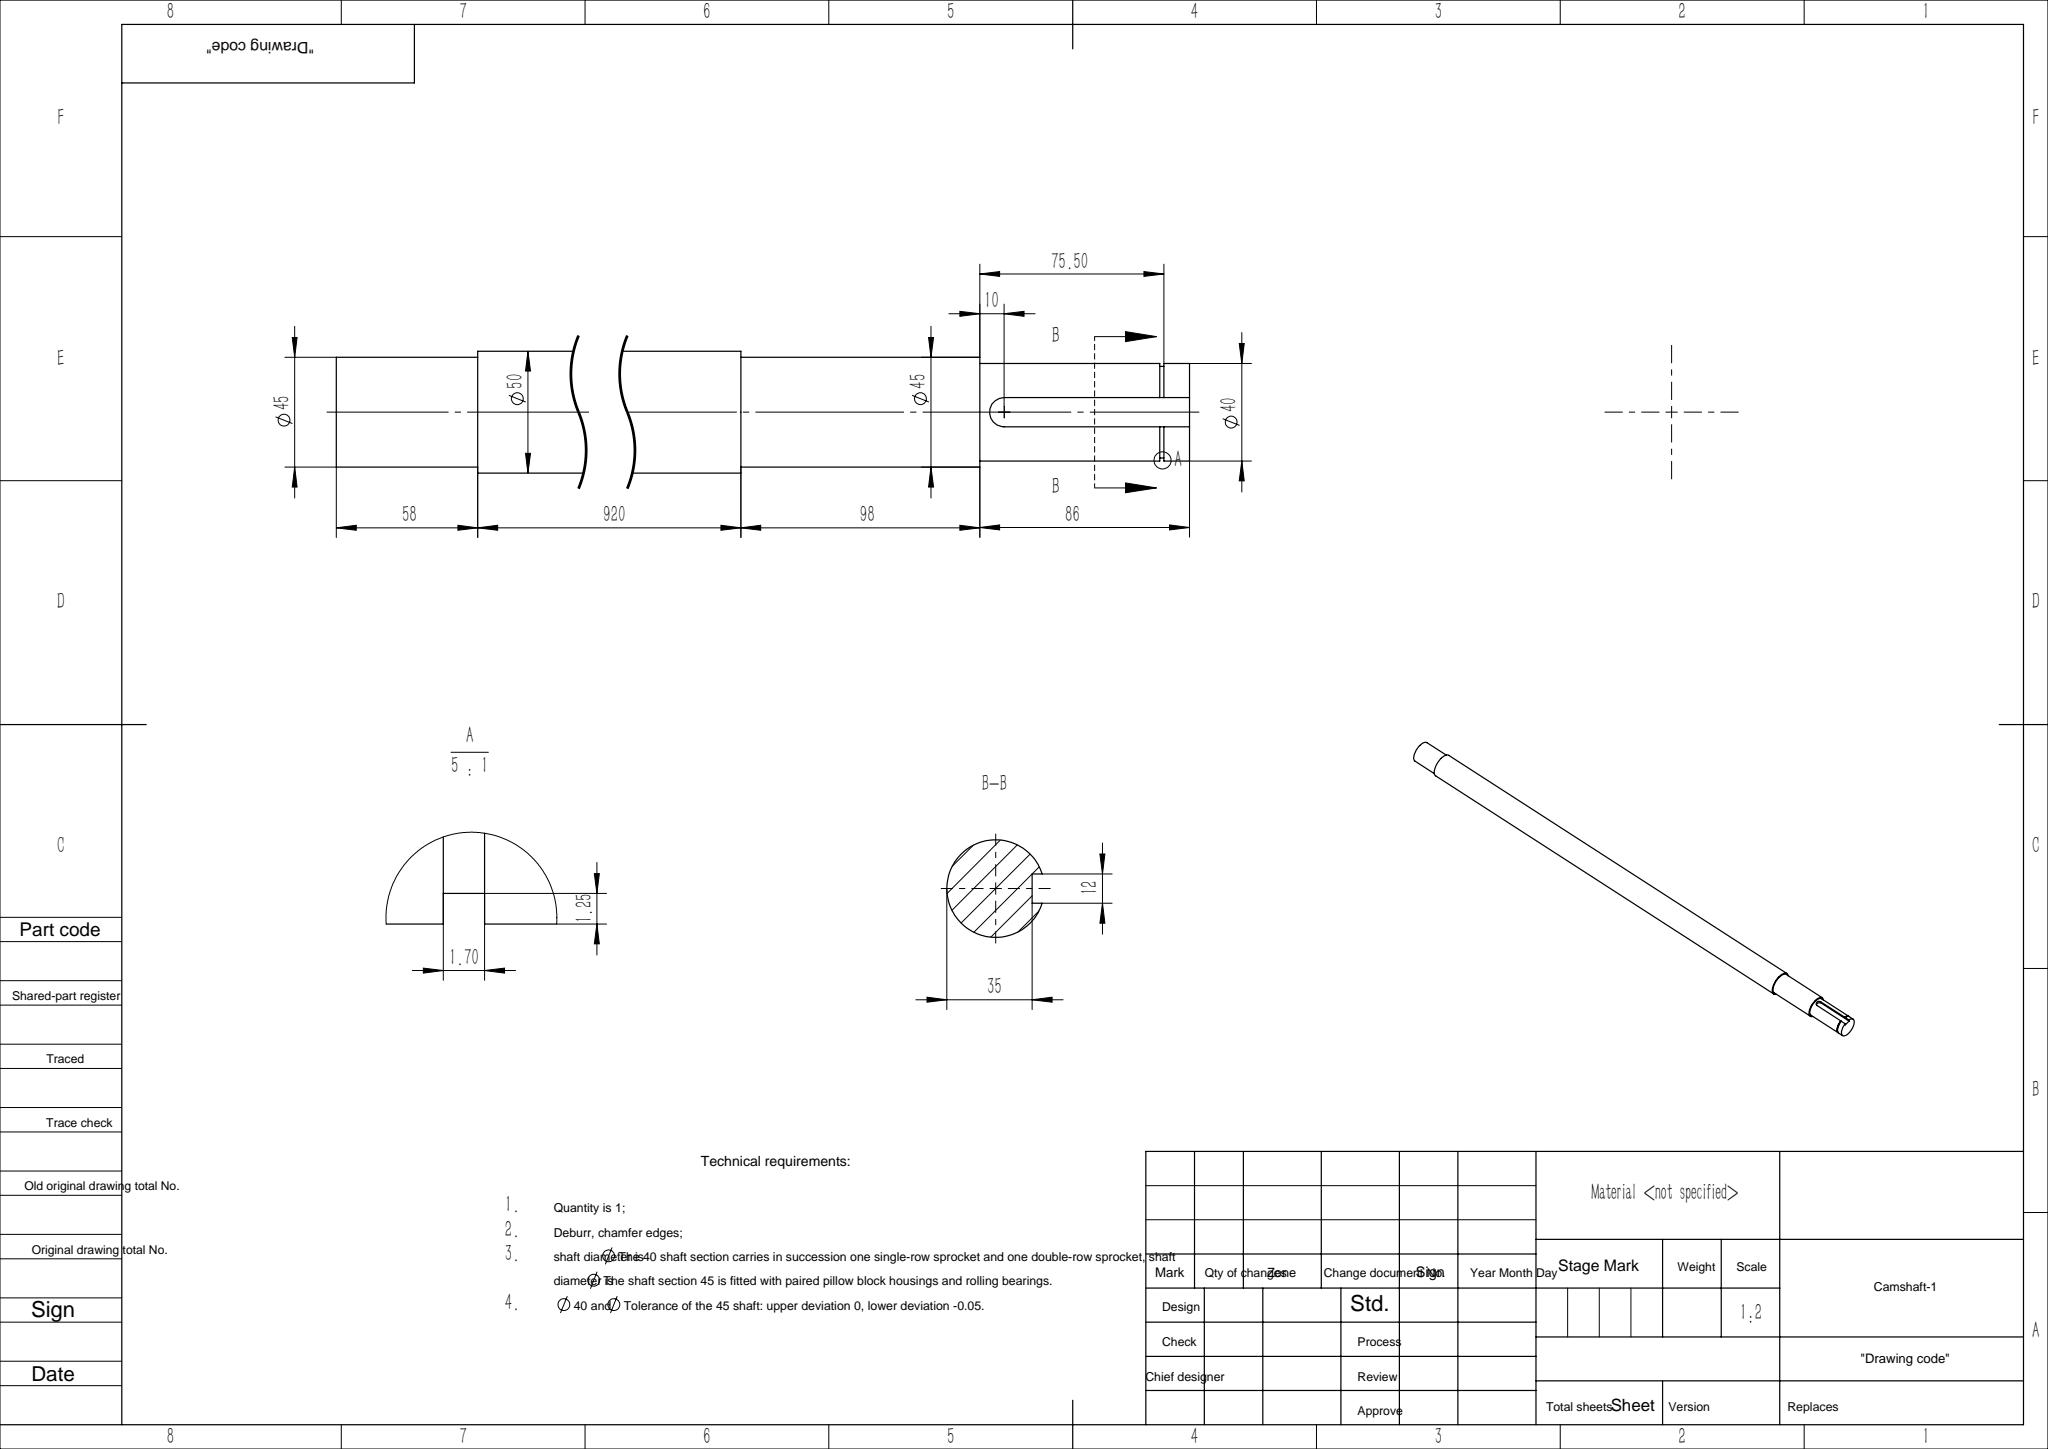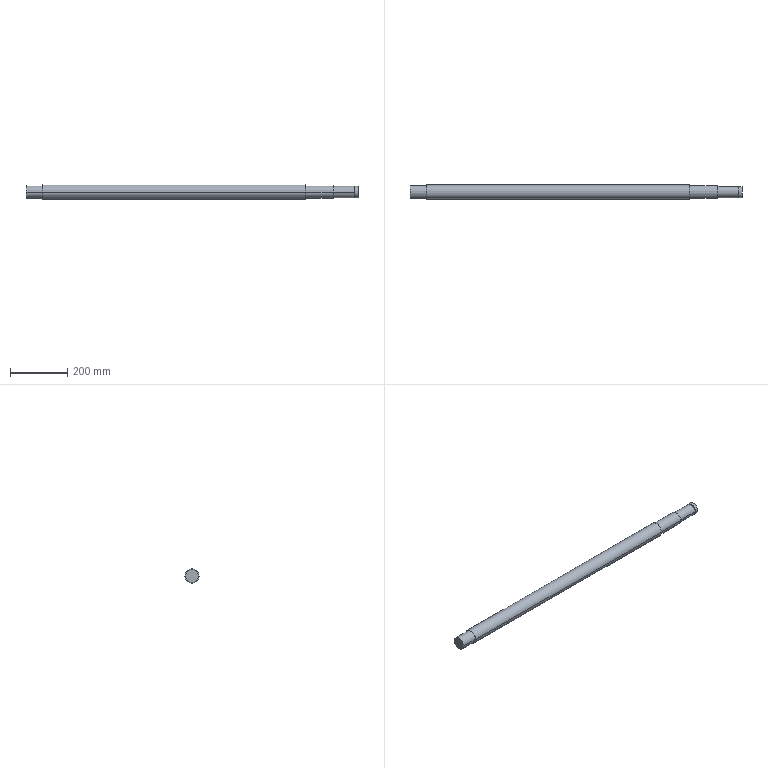Part | SolidWorks | features ICE 2, Revolution 1 | 1 solid | 22 faces | box 1162 x 50 x 50 mm | volume 2157809 mm3 | cylinder 12 | plane 10 | commonest cylinder face diameters 45 x4 40 x3 12 x2 50 x2 37.5 x1
STEP:
#1=CARTESIAN_POINT('',(1080.,15.,0.));
#2=VERTEX_POINT('',#1);
#3=CARTESIAN_POINT('',(1086.,15.,6.));
#4=VERTEX_POINT('',#3);
#5=CARTESIAN_POINT('',(1086.,15.,0.));
#6=DIRECTION('',(0.,1.,0.));
#7=DIRECTION('',(-1.,0.,0.));
#8=AXIS2_PLACEMENT_3D('',#5,#6,#7);
#9=CIRCLE('',#8,6.);
#10=EDGE_CURVE('',#2,#4,#9,.T.);
#11=ORIENTED_EDGE('',*,*,#10,.F.);
#12=CARTESIAN_POINT('',(1080.,20.,0.));
#13=VERTEX_POINT('',#12);
#14=CARTESIAN_POINT('',(1080.,15.,0.));
#15=DIRECTION('',(0.,1.,0.));
#16=VECTOR('',#15,1000.);
#17=LINE('',#14,#16);
#18=EDGE_CURVE('',#2,#13,#17,.T.);
#19=ORIENTED_EDGE('',*,*,#18,.T.);
#20=CARTESIAN_POINT('',(1086.,19.079,6.));
#21=VERTEX_POINT('',#20);
#22=CARTESIAN_POINT('',(1080.,20.,0.));
#23=CARTESIAN_POINT('',(1080.,20.,0.3936));
#24=CARTESIAN_POINT('',(1080.04,19.988,0.7934));
#25=CARTESIAN_POINT('',(1080.194,19.942,1.564));
#26=CARTESIAN_POINT('',(1080.308,19.909,1.939));
#27=CARTESIAN_POINT('',(1080.611,19.825,2.668));
#28=CARTESIAN_POINT('',(1080.798,19.774,3.015));
#29=CARTESIAN_POINT('',(1081.123,19.692,3.5));
#30=CARTESIAN_POINT('',(1081.239,19.664,3.657));
#31=CARTESIAN_POINT('',(1081.487,19.605,3.959));
#32=CARTESIAN_POINT('',(1081.62,19.575,4.105));
#33=CARTESIAN_POINT('',(1082.035,19.485,4.52));
#34=CARTESIAN_POINT('',(1082.335,19.425,4.766));
#35=CARTESIAN_POINT('',(1082.982,19.313,5.201));
#36=CARTESIAN_POINT('',(1083.333,19.261,5.389));
#37=CARTESIAN_POINT('',(1084.055,19.174,5.69));
#38=CARTESIAN_POINT('',(1084.429,19.139,5.804));
#39=CARTESIAN_POINT('',(1085.203,19.092,5.96));
#40=CARTESIAN_POINT('',(1085.601,19.079,6.));
#41=CARTESIAN_POINT('',(1086.,19.079,6.));
#42=B_SPLINE_CURVE_WITH_KNOTS('',3,(#22,#23,#24,#25,#26,#27,#28,#29,#30,#31,#32,#33,#34,#35,#36,#37,#38,#39,#40,#41),.UNSPECIFIED.,.F.,.F.,(4,2,2,2,2,2,2,2,2,4),(0.009436,0.01061,0.01179,0.01297,0.01356,0.01415,0.01533,0.0165,0.01768,0.01886),.UNSPECIFIED.);
#43=EDGE_CURVE('',#13,#21,#42,.T.);
#44=ORIENTED_EDGE('',*,*,#43,.T.);
#45=CARTESIAN_POINT('',(1086.,15.,6.));
#46=DIRECTION('',(0.,1.,0.));
#47=VECTOR('',#46,1000.);
#48=LINE('',#45,#47);
#49=EDGE_CURVE('',#4,#21,#48,.T.);
#50=ORIENTED_EDGE('',*,*,#49,.F.);
#51=EDGE_LOOP('',(#11,#19,#44,#50));
#52=FACE_OUTER_BOUND('',#51,.T.);
#53=CARTESIAN_POINT('',(1086.,15.,0.));
#54=DIRECTION('',(0.,1.,0.));
#55=DIRECTION('',(-1.,0.,0.));
#56=AXIS2_PLACEMENT_3D('',#53,#54,#55);
#57=CYLINDRICAL_SURFACE('',#56,6.);
#58=ADVANCED_FACE('',(#52),#57,.F.);
#59=CARTESIAN_POINT('',(978.,22.5,0.));
#60=VERTEX_POINT('',#59);
#61=CARTESIAN_POINT('',(978.,-22.5,0.));
#62=VERTEX_POINT('',#61);
#63=CARTESIAN_POINT('',(978.,0.,0.));
#64=DIRECTION('',(1.,0.,0.));
#65=DIRECTION('',(0.,1.,0.));
#66=AXIS2_PLACEMENT_3D('',#63,#64,#65);
#67=CIRCLE('',#66,22.5);
#68=EDGE_CURVE('',#60,#62,#67,.T.);
#69=ORIENTED_EDGE('',*,*,#68,.T.);
#70=CARTESIAN_POINT('',(1076.,-22.5,0.));
#71=VERTEX_POINT('',#70);
#72=CARTESIAN_POINT('',(1162.,-22.5,0.));
#73=DIRECTION('',(1.,0.,0.));
#74=VECTOR('',#73,1000.);
#75=LINE('',#72,#74);
#76=EDGE_CURVE('',#62,#71,#75,.T.);
#77=ORIENTED_EDGE('',*,*,#76,.T.);
#78=CARTESIAN_POINT('',(1076.,22.5,0.));
#79=VERTEX_POINT('',#78);
#80=CARTESIAN_POINT('',(1076.,0.,0.));
#81=DIRECTION('',(1.,0.,0.));
#82=DIRECTION('',(0.,1.,0.));
#83=AXIS2_PLACEMENT_3D('',#80,#81,#82);
#84=CIRCLE('',#83,22.5);
#85=EDGE_CURVE('',#79,#71,#84,.T.);
#86=ORIENTED_EDGE('',*,*,#85,.F.);
#87=CARTESIAN_POINT('',(1162.,22.5,0.));
#88=DIRECTION('',(1.,0.,0.));
#89=VECTOR('',#88,1000.);
#90=LINE('',#87,#89);
#91=EDGE_CURVE('',#60,#79,#90,.T.);
#92=ORIENTED_EDGE('',*,*,#91,.F.);
#93=EDGE_LOOP('',(#69,#77,#86,#92));
#94=FACE_OUTER_BOUND('',#93,.T.);
#95=CARTESIAN_POINT('',(1162.,0.,0.));
#96=DIRECTION('',(1.,0.,0.));
#97=DIRECTION('',(0.,1.,0.));
#98=AXIS2_PLACEMENT_3D('',#95,#96,#97);
#99=CYLINDRICAL_SURFACE('',#98,22.5);
#100=ADVANCED_FACE('',(#94),#99,.T.);
#101=CARTESIAN_POINT('',(58.,25.,0.));
#102=VERTEX_POINT('',#101);
#103=CARTESIAN_POINT('',(58.,-25.,0.));
#104=VERTEX_POINT('',#103);
#105=CARTESIAN_POINT('',(58.,0.,0.));
#106=DIRECTION('',(1.,0.,0.));
#107=DIRECTION('',(0.,1.,0.));
#108=AXIS2_PLACEMENT_3D('',#105,#106,#107);
#109=CIRCLE('',#108,25.);
#110=EDGE_CURVE('',#102,#104,#109,.T.);
#111=ORIENTED_EDGE('',*,*,#110,.T.);
#112=CARTESIAN_POINT('',(978.,-25.,0.));
#113=VERTEX_POINT('',#112);
#114=CARTESIAN_POINT('',(1162.,-25.,0.));
#115=DIRECTION('',(1.,0.,0.));
#116=VECTOR('',#115,1000.);
#117=LINE('',#114,#116);
#118=EDGE_CURVE('',#104,#113,#117,.T.);
#119=ORIENTED_EDGE('',*,*,#118,.T.);
#120=CARTESIAN_POINT('',(978.,25.,0.));
#121=VERTEX_POINT('',#120);
#122=CARTESIAN_POINT('',(978.,0.,0.));
#123=DIRECTION('',(1.,0.,0.));
#124=DIRECTION('',(0.,1.,0.));
#125=AXIS2_PLACEMENT_3D('',#122,#123,#124);
#126=CIRCLE('',#125,25.);
#127=EDGE_CURVE('',#121,#113,#126,.T.);
#128=ORIENTED_EDGE('',*,*,#127,.F.);
#129=CARTESIAN_POINT('',(1162.,25.,0.));
#130=DIRECTION('',(1.,0.,0.));
#131=VECTOR('',#130,1000.);
#132=LINE('',#129,#131);
#133=EDGE_CURVE('',#102,#121,#132,.T.);
#134=ORIENTED_EDGE('',*,*,#133,.F.);
#135=EDGE_LOOP('',(#111,#119,#128,#134));
#136=FACE_OUTER_BOUND('',#135,.T.);
#137=CARTESIAN_POINT('',(1162.,0.,0.));
#138=DIRECTION('',(1.,0.,0.));
#139=DIRECTION('',(0.,1.,0.));
#140=AXIS2_PLACEMENT_3D('',#137,#138,#139);
#141=CYLINDRICAL_SURFACE('',#140,25.);
#142=ADVANCED_FACE('',(#136),#141,.T.);
#143=CARTESIAN_POINT('',(0.,22.5,0.));
#144=VERTEX_POINT('',#143);
#145=CARTESIAN_POINT('',(0.,-22.5,0.));
#146=VERTEX_POINT('',#145);
#147=CARTESIAN_POINT('',(0.,0.,0.));
#148=DIRECTION('',(1.,0.,0.));
#149=DIRECTION('',(0.,1.,0.));
#150=AXIS2_PLACEMENT_3D('',#147,#148,#149);
#151=CIRCLE('',#150,22.5);
#152=EDGE_CURVE('',#144,#146,#151,.T.);
#153=ORIENTED_EDGE('',*,*,#152,.T.);
#154=CARTESIAN_POINT('',(58.,-22.5,0.));
#155=VERTEX_POINT('',#154);
#156=CARTESIAN_POINT('',(1162.,-22.5,0.));
#157=DIRECTION('',(1.,0.,0.));
#158=VECTOR('',#157,1000.);
#159=LINE('',#156,#158);
#160=EDGE_CURVE('',#146,#155,#159,.T.);
#161=ORIENTED_EDGE('',*,*,#160,.T.);
#162=CARTESIAN_POINT('',(58.,22.5,0.));
#163=VERTEX_POINT('',#162);
#164=CARTESIAN_POINT('',(58.,0.,0.));
#165=DIRECTION('',(1.,0.,0.));
#166=DIRECTION('',(0.,1.,0.));
#167=AXIS2_PLACEMENT_3D('',#164,#165,#166);
#168=CIRCLE('',#167,22.5);
#169=EDGE_CURVE('',#163,#155,#168,.T.);
#170=ORIENTED_EDGE('',*,*,#169,.F.);
#171=CARTESIAN_POINT('',(1162.,22.5,0.));
#172=DIRECTION('',(1.,0.,0.));
#173=VECTOR('',#172,1000.);
#174=LINE('',#171,#173);
#175=EDGE_CURVE('',#144,#163,#174,.T.);
#176=ORIENTED_EDGE('',*,*,#175,.F.);
#177=EDGE_LOOP('',(#153,#161,#170,#176));
#178=FACE_OUTER_BOUND('',#177,.T.);
#179=CARTESIAN_POINT('',(1162.,0.,0.));
#180=DIRECTION('',(1.,0.,0.));
#181=DIRECTION('',(0.,1.,0.));
#182=AXIS2_PLACEMENT_3D('',#179,#180,#181);
#183=CYLINDRICAL_SURFACE('',#182,22.5);
#184=ADVANCED_FACE('',(#178),#183,.T.);
#185=CARTESIAN_POINT('',(1076.,20.,0.));
#186=VERTEX_POINT('',#185);
#187=CARTESIAN_POINT('',(1076.,-20.,0.));
#188=VERTEX_POINT('',#187);
#189=CARTESIAN_POINT('',(1076.,0.,0.));
#190=DIRECTION('',(1.,0.,0.));
#191=DIRECTION('',(0.,1.,0.));
#192=AXIS2_PLACEMENT_3D('',#189,#190,#191);
#193=CIRCLE('',#192,20.);
#194=EDGE_CURVE('',#186,#188,#193,.T.);
#195=ORIENTED_EDGE('',*,*,#194,.T.);
#196=CARTESIAN_POINT('',(1149.8,-20.,0.));
#197=VERTEX_POINT('',#196);
#198=CARTESIAN_POINT('',(1162.,-20.,0.));
#199=DIRECTION('',(1.,0.,0.));
#200=VECTOR('',#199,1000.);
#201=LINE('',#198,#200);
#202=EDGE_CURVE('',#188,#197,#201,.T.);
#203=ORIENTED_EDGE('',*,*,#202,.T.);
#204=CARTESIAN_POINT('',(1149.8,19.079,6.));
#205=VERTEX_POINT('',#204);
#206=CARTESIAN_POINT('',(1149.8,0.,0.));
#207=DIRECTION('',(1.,0.,0.));
#208=DIRECTION('',(0.,1.,0.));
#209=AXIS2_PLACEMENT_3D('',#206,#207,#208);
#210=CIRCLE('',#209,20.);
#211=EDGE_CURVE('',#205,#197,#210,.T.);
#212=ORIENTED_EDGE('',*,*,#211,.F.);
#213=CARTESIAN_POINT('',(1162.,19.079,6.));
#214=DIRECTION('',(1.,0.,0.));
#215=VECTOR('',#214,1000.);
#216=LINE('',#213,#215);
#217=EDGE_CURVE('',#21,#205,#216,.T.);
#218=ORIENTED_EDGE('',*,*,#217,.F.);
#219=ORIENTED_EDGE('',*,*,#43,.F.);
#220=CARTESIAN_POINT('',(1162.,20.,0.));
#221=DIRECTION('',(1.,0.,0.));
#222=VECTOR('',#221,1000.);
#223=LINE('',#220,#222);
#224=EDGE_CURVE('',#186,#13,#223,.T.);
#225=ORIENTED_EDGE('',*,*,#224,.F.);
#226=EDGE_LOOP('',(#195,#203,#212,#218,#219,#225));
#227=FACE_OUTER_BOUND('',#226,.T.);
#228=CARTESIAN_POINT('',(1162.,0.,0.));
#229=DIRECTION('',(1.,0.,0.));
#230=DIRECTION('',(0.,1.,0.));
#231=AXIS2_PLACEMENT_3D('',#228,#229,#230);
#232=CYLINDRICAL_SURFACE('',#231,20.);
#233=ADVANCED_FACE('',(#227),#232,.T.);
#234=ORIENTED_EDGE('',*,*,#202,.F.);
#235=CARTESIAN_POINT('',(1076.,0.,0.));
#236=DIRECTION('',(1.,0.,0.));
#237=DIRECTION('',(0.,1.,0.));
#238=AXIS2_PLACEMENT_3D('',#235,#236,#237);
#239=CIRCLE('',#238,20.);
#240=EDGE_CURVE('',#188,#186,#239,.T.);
#241=ORIENTED_EDGE('',*,*,#240,.T.);
#242=ORIENTED_EDGE('',*,*,#224,.T.);
#243=CARTESIAN_POINT('',(1086.,19.079,-6.));
#244=VERTEX_POINT('',#243);
#245=CARTESIAN_POINT('',(1086.,19.079,-6.));
#246=CARTESIAN_POINT('',(1085.601,19.079,-6.));
#247=CARTESIAN_POINT('',(1085.209,19.091,-5.961));
#248=CARTESIAN_POINT('',(1084.631,19.127,-5.845));
#249=CARTESIAN_POINT('',(1084.441,19.141,-5.797));
#250=CARTESIAN_POINT('',(1084.062,19.176,-5.682));
#251=CARTESIAN_POINT('',(1083.875,19.196,-5.615));
#252=CARTESIAN_POINT('',(1083.331,19.261,-5.388));
#253=CARTESIAN_POINT('',(1082.987,19.313,-5.203));
#254=CARTESIAN_POINT('',(1082.499,19.397,-4.877));
#255=CARTESIAN_POINT('',(1082.34,19.426,-4.759));
#256=CARTESIAN_POINT('',(1082.037,19.485,-4.51));
#257=CARTESIAN_POINT('',(1081.893,19.515,-4.378));
#258=CARTESIAN_POINT('',(1081.481,19.605,-3.966));
#259=CARTESIAN_POINT('',(1081.233,19.664,-3.665));
#260=CARTESIAN_POINT('',(1080.794,19.775,-3.009));
#261=CARTESIAN_POINT('',(1080.609,19.825,-2.664));
#262=CARTESIAN_POINT('',(1080.385,19.888,-2.122));
#263=CARTESIAN_POINT('',(1080.318,19.907,-1.938));
#264=CARTESIAN_POINT('',(1080.203,19.94,-1.561));
#265=CARTESIAN_POINT('',(1080.154,19.954,-1.367));
#266=CARTESIAN_POINT('',(1080.038,19.988,-0.7852));
#267=CARTESIAN_POINT('',(1080.,20.,-0.3941));
#268=CARTESIAN_POINT('',(1080.,20.,0.));
#269=B_SPLINE_CURVE_WITH_KNOTS('',3,(#245,#246,#247,#248,#249,#250,#251,#252,#253,#254,#255,#256,#257,#258,#259,#260,#261,#262,#263,#264,#265,#266,#267,#268),.UNSPECIFIED.,.F.,.F.,(4,2,2,2,2,2,2,2,2,2,2,4),(0.,0.00118,0.001769,0.002359,0.003539,0.004128,0.004718,0.005898,0.007077,0.007667,0.008257,0.009436),.UNSPECIFIED.);
#270=EDGE_CURVE('',#244,#13,#269,.T.);
#271=ORIENTED_EDGE('',*,*,#270,.F.);
#272=CARTESIAN_POINT('',(1149.8,19.079,-6.));
#273=VERTEX_POINT('',#272);
#274=CARTESIAN_POINT('',(1162.,19.079,-6.));
#275=DIRECTION('',(-1.,0.,0.));
#276=VECTOR('',#275,1000.);
#277=LINE('',#274,#276);
#278=EDGE_CURVE('',#273,#244,#277,.T.);
#279=ORIENTED_EDGE('',*,*,#278,.F.);
#280=CARTESIAN_POINT('',(1149.8,0.,0.));
#281=DIRECTION('',(1.,0.,0.));
#282=DIRECTION('',(0.,1.,0.));
#283=AXIS2_PLACEMENT_3D('',#280,#281,#282);
#284=CIRCLE('',#283,20.);
#285=EDGE_CURVE('',#197,#273,#284,.T.);
#286=ORIENTED_EDGE('',*,*,#285,.F.);
#287=EDGE_LOOP('',(#234,#241,#242,#271,#279,#286));
#288=FACE_OUTER_BOUND('',#287,.T.);
#289=CARTESIAN_POINT('',(1162.,0.,0.));
#290=DIRECTION('',(1.,0.,0.));
#291=DIRECTION('',(0.,1.,0.));
#292=AXIS2_PLACEMENT_3D('',#289,#290,#291);
#293=CYLINDRICAL_SURFACE('',#292,20.);
#294=ADVANCED_FACE('',(#288),#293,.T.);
#295=CARTESIAN_POINT('',(1149.8,17.764,-6.));
#296=VERTEX_POINT('',#295);
#297=CARTESIAN_POINT('',(1149.8,15.,-6.));
#298=DIRECTION('',(0.,-1.,0.));
#299=VECTOR('',#298,1000.);
#300=LINE('',#297,#299);
#301=EDGE_CURVE('',#273,#296,#300,.T.);
#302=ORIENTED_EDGE('',*,*,#301,.F.);
#303=ORIENTED_EDGE('',*,*,#278,.T.);
#304=CARTESIAN_POINT('',(1086.,15.,-6.));
#305=VERTEX_POINT('',#304);
#306=CARTESIAN_POINT('',(1086.,15.,-6.));
#307=DIRECTION('',(0.,1.,0.));
#308=VECTOR('',#307,1000.);
#309=LINE('',#306,#308);
#310=EDGE_CURVE('',#305,#244,#309,.T.);
#311=ORIENTED_EDGE('',*,*,#310,.F.);
#312=CARTESIAN_POINT('',(1162.,15.,-6.));
#313=VERTEX_POINT('',#312);
#314=CARTESIAN_POINT('',(1086.,15.,-6.));
#315=DIRECTION('',(-1.,0.,0.));
#316=VECTOR('',#315,1000.);
#317=LINE('',#314,#316);
#318=EDGE_CURVE('',#313,#305,#317,.T.);
#319=ORIENTED_EDGE('',*,*,#318,.F.);
#320=CARTESIAN_POINT('',(1162.,19.079,-6.));
#321=VERTEX_POINT('',#320);
#322=CARTESIAN_POINT('',(1162.,20.,-6.));
#323=DIRECTION('',(0.,1.,0.));
#324=VECTOR('',#323,1000.);
#325=LINE('',#322,#324);
#326=EDGE_CURVE('',#313,#321,#325,.T.);
#327=ORIENTED_EDGE('',*,*,#326,.T.);
#328=CARTESIAN_POINT('',(1151.5,19.079,-6.));
#329=VERTEX_POINT('',#328);
#330=CARTESIAN_POINT('',(1162.,19.079,-6.));
#331=DIRECTION('',(-1.,0.,0.));
#332=VECTOR('',#331,1000.);
#333=LINE('',#330,#332);
#334=EDGE_CURVE('',#321,#329,#333,.T.);
#335=ORIENTED_EDGE('',*,*,#334,.T.);
#336=CARTESIAN_POINT('',(1151.5,17.764,-6.));
#337=VERTEX_POINT('',#336);
#338=CARTESIAN_POINT('',(1151.5,15.,-6.));
#339=DIRECTION('',(0.,-1.,0.));
#340=VECTOR('',#339,1000.);
#341=LINE('',#338,#340);
#342=EDGE_CURVE('',#329,#337,#341,.T.);
#343=ORIENTED_EDGE('',*,*,#342,.T.);
#344=CARTESIAN_POINT('',(1149.8,17.764,-6.));
#345=DIRECTION('',(1.,0.,0.));
#346=VECTOR('',#345,1000.);
#347=LINE('',#344,#346);
#348=EDGE_CURVE('',#296,#337,#347,.T.);
#349=ORIENTED_EDGE('',*,*,#348,.F.);
#350=EDGE_LOOP('',(#302,#303,#311,#319,#327,#335,#343,#349));
#351=FACE_OUTER_BOUND('',#350,.T.);
#352=CARTESIAN_POINT('',(1086.,15.,-6.));
#353=DIRECTION('',(0.,0.,-1.));
#354=DIRECTION('',(-1.,0.,0.));
#355=AXIS2_PLACEMENT_3D('',#352,#353,#354);
#356=PLANE('',#355);
#357=ADVANCED_FACE('',(#351),#356,.F.);
#358=CARTESIAN_POINT('',(1149.8,17.764,6.));
#359=VERTEX_POINT('',#358);
#360=CARTESIAN_POINT('',(1149.8,15.,6.));
#361=DIRECTION('',(0.,1.,0.));
#362=VECTOR('',#361,1000.);
#363=LINE('',#360,#362);
#364=EDGE_CURVE('',#359,#205,#363,.T.);
#365=ORIENTED_EDGE('',*,*,#364,.F.);
#366=CARTESIAN_POINT('',(1151.5,17.764,6.));
#367=VERTEX_POINT('',#366);
#368=CARTESIAN_POINT('',(1149.8,17.764,6.));
#369=DIRECTION('',(-1.,0.,0.));
#370=VECTOR('',#369,1000.);
#371=LINE('',#368,#370);
#372=EDGE_CURVE('',#367,#359,#371,.T.);
#373=ORIENTED_EDGE('',*,*,#372,.F.);
#374=CARTESIAN_POINT('',(1151.5,19.079,6.));
#375=VERTEX_POINT('',#374);
#376=CARTESIAN_POINT('',(1151.5,15.,6.));
#377=DIRECTION('',(0.,1.,0.));
#378=VECTOR('',#377,1000.);
#379=LINE('',#376,#378);
#380=EDGE_CURVE('',#367,#375,#379,.T.);
#381=ORIENTED_EDGE('',*,*,#380,.T.);
#382=CARTESIAN_POINT('',(1162.,19.079,6.));
#383=VERTEX_POINT('',#382);
#384=CARTESIAN_POINT('',(1162.,19.079,6.));
#385=DIRECTION('',(1.,0.,0.));
#386=VECTOR('',#385,1000.);
#387=LINE('',#384,#386);
#388=EDGE_CURVE('',#375,#383,#387,.T.);
#389=ORIENTED_EDGE('',*,*,#388,.T.);
#390=CARTESIAN_POINT('',(1162.,15.,6.));
#391=VERTEX_POINT('',#390);
#392=CARTESIAN_POINT('',(1162.,20.,6.));
#393=DIRECTION('',(0.,-1.,0.));
#394=VECTOR('',#393,1000.);
#395=LINE('',#392,#394);
#396=EDGE_CURVE('',#383,#391,#395,.T.);
#397=ORIENTED_EDGE('',*,*,#396,.T.);
#398=CARTESIAN_POINT('',(1172.,15.,6.));
#399=DIRECTION('',(1.,0.,0.));
#400=VECTOR('',#399,1000.);
#401=LINE('',#398,#400);
#402=EDGE_CURVE('',#4,#391,#401,.T.);
#403=ORIENTED_EDGE('',*,*,#402,.F.);
#404=ORIENTED_EDGE('',*,*,#49,.T.);
#405=ORIENTED_EDGE('',*,*,#217,.T.);
#406=EDGE_LOOP('',(#365,#373,#381,#389,#397,#403,#404,#405));
#407=FACE_OUTER_BOUND('',#406,.T.);
#408=CARTESIAN_POINT('',(1172.,15.,6.));
#409=DIRECTION('',(0.,0.,1.));
#410=DIRECTION('',(1.,0.,0.));
#411=AXIS2_PLACEMENT_3D('',#408,#409,#410);
#412=PLANE('',#411);
#413=ADVANCED_FACE('',(#407),#412,.F.);
#414=ORIENTED_EDGE('',*,*,#152,.F.);
#415=CARTESIAN_POINT('',(0.,0.,0.));
#416=DIRECTION('',(1.,0.,0.));
#417=DIRECTION('',(0.,1.,0.));
#418=AXIS2_PLACEMENT_3D('',#415,#416,#417);
#419=CIRCLE('',#418,22.5);
#420=EDGE_CURVE('',#146,#144,#419,.T.);
#421=ORIENTED_EDGE('',*,*,#420,.F.);
#422=EDGE_LOOP('',(#414,#421));
#423=FACE_OUTER_BOUND('',#422,.T.);
#424=CARTESIAN_POINT('',(0.,0.,0.));
#425=DIRECTION('',(-1.,0.,0.));
#426=DIRECTION('',(0.,-1.,0.));
#427=AXIS2_PLACEMENT_3D('',#424,#425,#426);
#428=PLANE('',#427);
#429=ADVANCED_FACE('',(#423),#428,.T.);
#430=ORIENTED_EDGE('',*,*,#160,.F.);
#431=ORIENTED_EDGE('',*,*,#420,.T.);
#432=ORIENTED_EDGE('',*,*,#175,.T.);
#433=CARTESIAN_POINT('',(58.,0.,0.));
#434=DIRECTION('',(1.,0.,0.));
#435=DIRECTION('',(0.,1.,0.));
#436=AXIS2_PLACEMENT_3D('',#433,#434,#435);
#437=CIRCLE('',#436,22.5);
#438=EDGE_CURVE('',#155,#163,#437,.T.);
#439=ORIENTED_EDGE('',*,*,#438,.F.);
#440=EDGE_LOOP('',(#430,#431,#432,#439));
#441=FACE_OUTER_BOUND('',#440,.T.);
#442=CARTESIAN_POINT('',(1162.,0.,0.));
#443=DIRECTION('',(1.,0.,0.));
#444=DIRECTION('',(0.,1.,0.));
#445=AXIS2_PLACEMENT_3D('',#442,#443,#444);
#446=CYLINDRICAL_SURFACE('',#445,22.5);
#447=ADVANCED_FACE('',(#441),#446,.T.);
#448=ORIENTED_EDGE('',*,*,#169,.T.);
#449=ORIENTED_EDGE('',*,*,#438,.T.);
#450=EDGE_LOOP('',(#448,#449));
#451=FACE_BOUND('',#450,.T.);
#452=ORIENTED_EDGE('',*,*,#110,.F.);
#453=CARTESIAN_POINT('',(58.,0.,0.));
#454=DIRECTION('',(1.,0.,0.));
#455=DIRECTION('',(0.,1.,0.));
#456=AXIS2_PLACEMENT_3D('',#453,#454,#455);
#457=CIRCLE('',#456,25.);
#458=EDGE_CURVE('',#104,#102,#457,.T.);
#459=ORIENTED_EDGE('',*,*,#458,.F.);
#460=EDGE_LOOP('',(#452,#459));
#461=FACE_OUTER_BOUND('',#460,.T.);
#462=CARTESIAN_POINT('',(58.,22.5,0.));
#463=DIRECTION('',(-1.,0.,0.));
#464=DIRECTION('',(0.,-1.,0.));
#465=AXIS2_PLACEMENT_3D('',#462,#463,#464);
#466=PLANE('',#465);
#467=ADVANCED_FACE('',(#451,#461),#466,.T.);
#468=ORIENTED_EDGE('',*,*,#118,.F.);
#469=ORIENTED_EDGE('',*,*,#458,.T.);
#470=ORIENTED_EDGE('',*,*,#133,.T.);
#471=CARTESIAN_POINT('',(978.,0.,0.));
#472=DIRECTION('',(1.,0.,0.));
#473=DIRECTION('',(0.,1.,0.));
#474=AXIS2_PLACEMENT_3D('',#471,#472,#473);
#475=CIRCLE('',#474,25.);
#476=EDGE_CURVE('',#113,#121,#475,.T.);
#477=ORIENTED_EDGE('',*,*,#476,.F.);
#478=EDGE_LOOP('',(#468,#469,#470,#477));
#479=FACE_OUTER_BOUND('',#478,.T.);
#480=CARTESIAN_POINT('',(1162.,0.,0.));
#481=DIRECTION('',(1.,0.,0.));
#482=DIRECTION('',(0.,1.,0.));
#483=AXIS2_PLACEMENT_3D('',#480,#481,#482);
#484=CYLINDRICAL_SURFACE('',#483,25.);
#485=ADVANCED_FACE('',(#479),#484,.T.);
#486=ORIENTED_EDGE('',*,*,#127,.T.);
#487=ORIENTED_EDGE('',*,*,#476,.T.);
#488=EDGE_LOOP('',(#486,#487));
#489=FACE_OUTER_BOUND('',#488,.T.);
#490=ORIENTED_EDGE('',*,*,#68,.F.);
#491=CARTESIAN_POINT('',(978.,0.,0.));
#492=DIRECTION('',(1.,0.,0.));
#493=DIRECTION('',(0.,1.,0.));
#494=AXIS2_PLACEMENT_3D('',#491,#492,#493);
#495=CIRCLE('',#494,22.5);
#496=EDGE_CURVE('',#62,#60,#495,.T.);
#497=ORIENTED_EDGE('',*,*,#496,.F.);
#498=EDGE_LOOP('',(#490,#497));
#499=FACE_BOUND('',#498,.T.);
#500=CARTESIAN_POINT('',(978.,25.,0.));
#501=DIRECTION('',(1.,0.,0.));
#502=DIRECTION('',(0.,1.,0.));
#503=AXIS2_PLACEMENT_3D('',#500,#501,#502);
#504=PLANE('',#503);
#505=ADVANCED_FACE('',(#489,#499),#504,.T.);
#506=ORIENTED_EDGE('',*,*,#76,.F.);
#507=ORIENTED_EDGE('',*,*,#496,.T.);
#508=ORIENTED_EDGE('',*,*,#91,.T.);
#509=CARTESIAN_POINT('',(1076.,0.,0.));
#510=DIRECTION('',(1.,0.,0.));
#511=DIRECTION('',(0.,1.,0.));
#512=AXIS2_PLACEMENT_3D('',#509,#510,#511);
#513=CIRCLE('',#512,22.5);
#514=EDGE_CURVE('',#71,#79,#513,.T.);
#515=ORIENTED_EDGE('',*,*,#514,.F.);
#516=EDGE_LOOP('',(#506,#507,#508,#515));
#517=FACE_OUTER_BOUND('',#516,.T.);
#518=CARTESIAN_POINT('',(1162.,0.,0.));
#519=DIRECTION('',(1.,0.,0.));
#520=DIRECTION('',(0.,1.,0.));
#521=AXIS2_PLACEMENT_3D('',#518,#519,#520);
#522=CYLINDRICAL_SURFACE('',#521,22.5);
#523=ADVANCED_FACE('',(#517),#522,.T.);
#524=ORIENTED_EDGE('',*,*,#85,.T.);
#525=ORIENTED_EDGE('',*,*,#514,.T.);
#526=EDGE_LOOP('',(#524,#525));
#527=FACE_OUTER_BOUND('',#526,.T.);
#528=ORIENTED_EDGE('',*,*,#194,.F.);
#529=ORIENTED_EDGE('',*,*,#240,.F.);
#530=EDGE_LOOP('',(#528,#529));
#531=FACE_BOUND('',#530,.T.);
#532=CARTESIAN_POINT('',(1076.,22.5,0.));
#533=DIRECTION('',(1.,0.,0.));
#534=DIRECTION('',(0.,1.,0.));
#535=AXIS2_PLACEMENT_3D('',#532,#533,#534);
#536=PLANE('',#535);
#537=ADVANCED_FACE('',(#527,#531),#536,.T.);
#538=CARTESIAN_POINT('',(1151.5,0.,0.));
#539=DIRECTION('',(1.,0.,0.));
#540=DIRECTION('',(0.,1.,0.));
#541=AXIS2_PLACEMENT_3D('',#538,#539,#540);
#542=CIRCLE('',#541,20.);
#543=EDGE_CURVE('',#375,#329,#542,.T.);
#544=ORIENTED_EDGE('',*,*,#543,.T.);
#545=ORIENTED_EDGE('',*,*,#334,.F.);
#546=CARTESIAN_POINT('',(1162.,0.,0.));
#547=DIRECTION('',(1.,0.,0.));
#548=DIRECTION('',(0.,1.,0.));
#549=AXIS2_PLACEMENT_3D('',#546,#547,#548);
#550=CIRCLE('',#549,20.);
#551=EDGE_CURVE('',#383,#321,#550,.T.);
#552=ORIENTED_EDGE('',*,*,#551,.F.);
#553=ORIENTED_EDGE('',*,*,#388,.F.);
#554=EDGE_LOOP('',(#544,#545,#552,#553));
#555=FACE_OUTER_BOUND('',#554,.T.);
#556=CARTESIAN_POINT('',(1162.,0.,0.));
#557=DIRECTION('',(1.,0.,0.));
#558=DIRECTION('',(0.,1.,0.));
#559=AXIS2_PLACEMENT_3D('',#556,#557,#558);
#560=CYLINDRICAL_SURFACE('',#559,20.);
#561=ADVANCED_FACE('',(#555),#560,.T.);
#562=ORIENTED_EDGE('',*,*,#326,.F.);
#563=CARTESIAN_POINT('',(1162.,15.,0.));
#564=DIRECTION('',(0.,0.,1.));
#565=VECTOR('',#564,1000.);
#566=LINE('',#563,#565);
#567=EDGE_CURVE('',#313,#391,#566,.T.);
#568=ORIENTED_EDGE('',*,*,#567,.T.);
#569=ORIENTED_EDGE('',*,*,#396,.F.);
#570=ORIENTED_EDGE('',*,*,#551,.T.);
#571=EDGE_LOOP('',(#562,#568,#569,#570));
#572=FACE_OUTER_BOUND('',#571,.T.);
#573=CARTESIAN_POINT('',(1162.,20.,0.));
#574=DIRECTION('',(1.,0.,0.));
#575=DIRECTION('',(0.,1.,0.));
#576=AXIS2_PLACEMENT_3D('',#573,#574,#575);
#577=PLANE('',#576);
#578=ADVANCED_FACE('',(#572),#577,.T.);
#579=ORIENTED_EDGE('',*,*,#18,.F.);
#580=CARTESIAN_POINT('',(1086.,15.,0.));
#581=DIRECTION('',(0.,1.,0.));
#582=DIRECTION('',(-1.,0.,0.));
#583=AXIS2_PLACEMENT_3D('',#580,#581,#582);
#584=CIRCLE('',#583,6.);
#585=EDGE_CURVE('',#305,#2,#584,.T.);
#586=ORIENTED_EDGE('',*,*,#585,.F.);
#587=ORIENTED_EDGE('',*,*,#310,.T.);
#588=ORIENTED_EDGE('',*,*,#270,.T.);
#589=EDGE_LOOP('',(#579,#586,#587,#588));
#590=FACE_OUTER_BOUND('',#589,.T.);
#591=CARTESIAN_POINT('',(1086.,15.,0.));
#592=DIRECTION('',(0.,1.,0.));
#593=DIRECTION('',(-1.,0.,0.));
#594=AXIS2_PLACEMENT_3D('',#591,#592,#593);
#595=CYLINDRICAL_SURFACE('',#594,6.);
#596=ADVANCED_FACE('',(#590),#595,.F.);
#597=ORIENTED_EDGE('',*,*,#318,.T.);
#598=ORIENTED_EDGE('',*,*,#585,.T.);
#599=ORIENTED_EDGE('',*,*,#10,.T.);
#600=ORIENTED_EDGE('',*,*,#402,.T.);
#601=ORIENTED_EDGE('',*,*,#567,.F.);
#602=EDGE_LOOP('',(#597,#598,#599,#600,#601));
#603=FACE_OUTER_BOUND('',#602,.T.);
#604=CARTESIAN_POINT('',(1086.,15.,0.));
#605=DIRECTION('',(0.,1.,0.));
#606=DIRECTION('',(-1.,0.,0.));
#607=AXIS2_PLACEMENT_3D('',#604,#605,#606);
#608=PLANE('',#607);
#609=ADVANCED_FACE('',(#603),#608,.T.);
#610=ORIENTED_EDGE('',*,*,#301,.T.);
#611=CARTESIAN_POINT('',(1149.8,0.,0.));
#612=DIRECTION('',(1.,0.,0.));
#613=DIRECTION('',(0.,1.,0.));
#614=AXIS2_PLACEMENT_3D('',#611,#612,#613);
#615=CIRCLE('',#614,18.75);
#616=EDGE_CURVE('',#359,#296,#615,.T.);
#617=ORIENTED_EDGE('',*,*,#616,.F.);
#618=ORIENTED_EDGE('',*,*,#364,.T.);
#619=ORIENTED_EDGE('',*,*,#211,.T.);
#620=ORIENTED_EDGE('',*,*,#285,.T.);
#621=EDGE_LOOP('',(#610,#617,#618,#619,#620));
#622=FACE_OUTER_BOUND('',#621,.T.);
#623=CARTESIAN_POINT('',(1149.8,0.,0.));
#624=DIRECTION('',(1.,0.,0.));
#625=DIRECTION('',(0.,1.,0.));
#626=AXIS2_PLACEMENT_3D('',#623,#624,#625);
#627=PLANE('',#626);
#628=ADVANCED_FACE('',(#622),#627,.T.);
#629=ORIENTED_EDGE('',*,*,#543,.F.);
#630=ORIENTED_EDGE('',*,*,#380,.F.);
#631=CARTESIAN_POINT('',(1151.5,0.,0.));
#632=DIRECTION('',(1.,0.,0.));
#633=DIRECTION('',(0.,1.,0.));
#634=AXIS2_PLACEMENT_3D('',#631,#632,#633);
#635=CIRCLE('',#634,18.75);
#636=EDGE_CURVE('',#367,#337,#635,.T.);
#637=ORIENTED_EDGE('',*,*,#636,.T.);
#638=ORIENTED_EDGE('',*,*,#342,.F.);
#639=EDGE_LOOP('',(#629,#630,#637,#638));
#640=FACE_OUTER_BOUND('',#639,.T.);
#641=CARTESIAN_POINT('',(1151.5,0.,0.));
#642=DIRECTION('',(1.,0.,0.));
#643=DIRECTION('',(0.,1.,0.));
#644=AXIS2_PLACEMENT_3D('',#641,#642,#643);
#645=PLANE('',#644);
#646=ADVANCED_FACE('',(#640),#645,.F.);
#647=ORIENTED_EDGE('',*,*,#348,.T.);
#648=ORIENTED_EDGE('',*,*,#636,.F.);
#649=ORIENTED_EDGE('',*,*,#372,.T.);
#650=ORIENTED_EDGE('',*,*,#616,.T.);
#651=EDGE_LOOP('',(#647,#648,#649,#650));
#652=FACE_OUTER_BOUND('',#651,.T.);
#653=CARTESIAN_POINT('',(1149.8,0.,0.));
#654=DIRECTION('',(1.,0.,0.));
#655=DIRECTION('',(0.,1.,0.));
#656=AXIS2_PLACEMENT_3D('',#653,#654,#655);
#657=CYLINDRICAL_SURFACE('',#656,18.75);
#658=ADVANCED_FACE('',(#652),#657,.T.);
#659=CLOSED_SHELL('',(#58,#100,#142,#184,#233,#294,#357,#413,#429,#447,#467,#485,#505,#523,#537,#561,#578,#596,#609,#628,#646,#658));
#660=MANIFOLD_SOLID_BREP('',#659);
#661=CARTESIAN_POINT('',(0.,0.,0.));
#662=DIRECTION('',(0.,0.,1.));
#663=DIRECTION('',(1.,0.,0.));
#664=AXIS2_PLACEMENT_3D('',#661,#662,#663);
#665=(LENGTH_UNIT()NAMED_UNIT(*)SI_UNIT(.MILLI.,.METRE.));
#666=UNCERTAINTY_MEASURE_WITH_UNIT(LENGTH_MEASURE(0.00001),#665,'','');
#667=(NAMED_UNIT(*)PLANE_ANGLE_UNIT()SI_UNIT($,.RADIAN.));
#668=(NAMED_UNIT(*)SI_UNIT($,.STERADIAN.)SOLID_ANGLE_UNIT());
#669=(GEOMETRIC_REPRESENTATION_CONTEXT(3)GLOBAL_UNCERTAINTY_ASSIGNED_CONTEXT((#666))GLOBAL_UNIT_ASSIGNED_CONTEXT((#665,#667,#668))REPRESENTATION_CONTEXT('',''));
#670=ADVANCED_BREP_SHAPE_REPRESENTATION('',(#660,#664),#669);